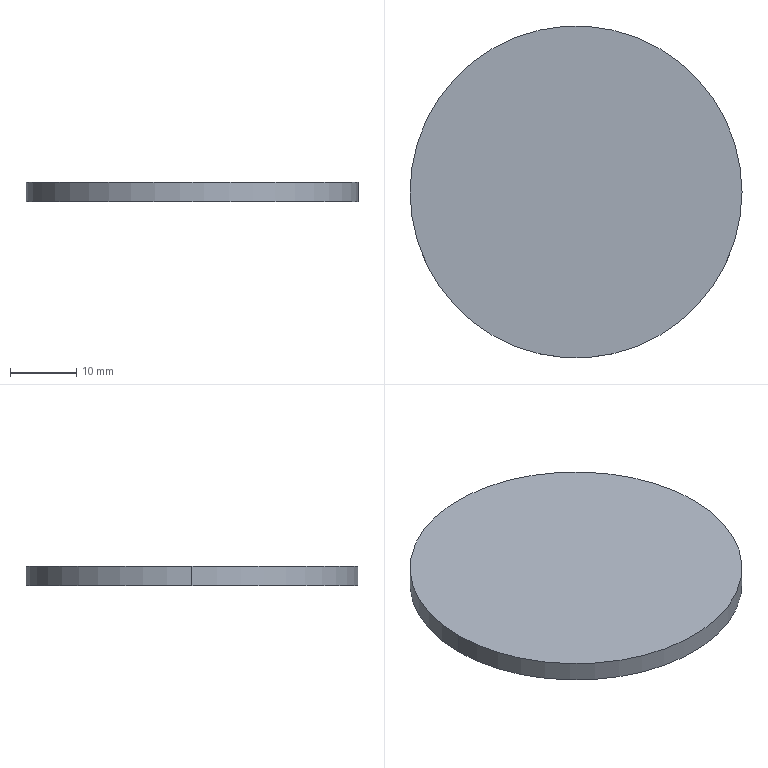Part | SolidWorks | features Extrusion 1 | 1 solid | 4 faces | box 50 x 50 x 3 mm | volume 5890 mm3 | cylinder 2 | plane 2 | commonest cylinder face diameters 50 x2
STEP:
#1=CARTESIAN_POINT('',(25.,0.,3.));
#2=VERTEX_POINT('',#1);
#3=CARTESIAN_POINT('',(-25.,0.,3.));
#4=VERTEX_POINT('',#3);
#5=CARTESIAN_POINT('',(0.,0.,3.));
#6=DIRECTION('',(0.,0.,1.));
#7=DIRECTION('',(1.,0.,0.));
#8=AXIS2_PLACEMENT_3D('',#5,#6,#7);
#9=CIRCLE('',#8,25.);
#10=EDGE_CURVE('',#2,#4,#9,.T.);
#11=ORIENTED_EDGE('',*,*,#10,.F.);
#12=CARTESIAN_POINT('',(25.,0.,0.));
#13=VERTEX_POINT('',#12);
#14=CARTESIAN_POINT('',(25.,0.,3.));
#15=DIRECTION('',(0.,0.,-1.));
#16=VECTOR('',#15,1000.);
#17=LINE('',#14,#16);
#18=EDGE_CURVE('',#2,#13,#17,.T.);
#19=ORIENTED_EDGE('',*,*,#18,.T.);
#20=CARTESIAN_POINT('',(-25.,0.,0.));
#21=VERTEX_POINT('',#20);
#22=CARTESIAN_POINT('',(0.,0.,0.));
#23=DIRECTION('',(0.,0.,1.));
#24=DIRECTION('',(1.,0.,0.));
#25=AXIS2_PLACEMENT_3D('',#22,#23,#24);
#26=CIRCLE('',#25,25.);
#27=EDGE_CURVE('',#13,#21,#26,.T.);
#28=ORIENTED_EDGE('',*,*,#27,.T.);
#29=CARTESIAN_POINT('',(-25.,0.,3.));
#30=DIRECTION('',(0.,0.,-1.));
#31=VECTOR('',#30,1000.);
#32=LINE('',#29,#31);
#33=EDGE_CURVE('',#4,#21,#32,.T.);
#34=ORIENTED_EDGE('',*,*,#33,.F.);
#35=EDGE_LOOP('',(#11,#19,#28,#34));
#36=FACE_OUTER_BOUND('',#35,.T.);
#37=CARTESIAN_POINT('',(0.,0.,3.));
#38=DIRECTION('',(0.,0.,-1.));
#39=DIRECTION('',(-1.,0.,0.));
#40=AXIS2_PLACEMENT_3D('',#37,#38,#39);
#41=CYLINDRICAL_SURFACE('',#40,25.);
#42=ADVANCED_FACE('',(#36),#41,.T.);
#43=ORIENTED_EDGE('',*,*,#18,.F.);
#44=CARTESIAN_POINT('',(0.,0.,3.));
#45=DIRECTION('',(0.,0.,1.));
#46=DIRECTION('',(1.,0.,0.));
#47=AXIS2_PLACEMENT_3D('',#44,#45,#46);
#48=CIRCLE('',#47,25.);
#49=EDGE_CURVE('',#4,#2,#48,.T.);
#50=ORIENTED_EDGE('',*,*,#49,.F.);
#51=ORIENTED_EDGE('',*,*,#33,.T.);
#52=CARTESIAN_POINT('',(0.,0.,0.));
#53=DIRECTION('',(0.,0.,1.));
#54=DIRECTION('',(1.,0.,0.));
#55=AXIS2_PLACEMENT_3D('',#52,#53,#54);
#56=CIRCLE('',#55,25.);
#57=EDGE_CURVE('',#21,#13,#56,.T.);
#58=ORIENTED_EDGE('',*,*,#57,.T.);
#59=EDGE_LOOP('',(#43,#50,#51,#58));
#60=FACE_OUTER_BOUND('',#59,.T.);
#61=CARTESIAN_POINT('',(0.,0.,3.));
#62=DIRECTION('',(0.,0.,-1.));
#63=DIRECTION('',(-1.,0.,0.));
#64=AXIS2_PLACEMENT_3D('',#61,#62,#63);
#65=CYLINDRICAL_SURFACE('',#64,25.);
#66=ADVANCED_FACE('',(#60),#65,.T.);
#67=ORIENTED_EDGE('',*,*,#49,.T.);
#68=ORIENTED_EDGE('',*,*,#10,.T.);
#69=EDGE_LOOP('',(#67,#68));
#70=FACE_OUTER_BOUND('',#69,.T.);
#71=CARTESIAN_POINT('',(0.,0.,3.));
#72=DIRECTION('',(0.,0.,1.));
#73=DIRECTION('',(1.,0.,0.));
#74=AXIS2_PLACEMENT_3D('',#71,#72,#73);
#75=PLANE('',#74);
#76=ADVANCED_FACE('',(#70),#75,.T.);
#77=ORIENTED_EDGE('',*,*,#57,.F.);
#78=ORIENTED_EDGE('',*,*,#27,.F.);
#79=EDGE_LOOP('',(#77,#78));
#80=FACE_OUTER_BOUND('',#79,.T.);
#81=CARTESIAN_POINT('',(0.,0.,0.));
#82=DIRECTION('',(0.,0.,1.));
#83=DIRECTION('',(1.,0.,0.));
#84=AXIS2_PLACEMENT_3D('',#81,#82,#83);
#85=PLANE('',#84);
#86=ADVANCED_FACE('',(#80),#85,.F.);
#87=CLOSED_SHELL('',(#42,#66,#76,#86));
#88=MANIFOLD_SOLID_BREP('',#87);
#89=CARTESIAN_POINT('',(0.,0.,0.));
#90=DIRECTION('',(0.,0.,1.));
#91=DIRECTION('',(1.,0.,0.));
#92=AXIS2_PLACEMENT_3D('',#89,#90,#91);
#93=(LENGTH_UNIT()NAMED_UNIT(*)SI_UNIT(.MILLI.,.METRE.));
#94=UNCERTAINTY_MEASURE_WITH_UNIT(LENGTH_MEASURE(0.00001),#93,'','');
#95=(NAMED_UNIT(*)PLANE_ANGLE_UNIT()SI_UNIT($,.RADIAN.));
#96=(NAMED_UNIT(*)SI_UNIT($,.STERADIAN.)SOLID_ANGLE_UNIT());
#97=(GEOMETRIC_REPRESENTATION_CONTEXT(3)GLOBAL_UNCERTAINTY_ASSIGNED_CONTEXT((#94))GLOBAL_UNIT_ASSIGNED_CONTEXT((#93,#95,#96))REPRESENTATION_CONTEXT('',''));
#98=ADVANCED_BREP_SHAPE_REPRESENTATION('',(#88,#92),#97);